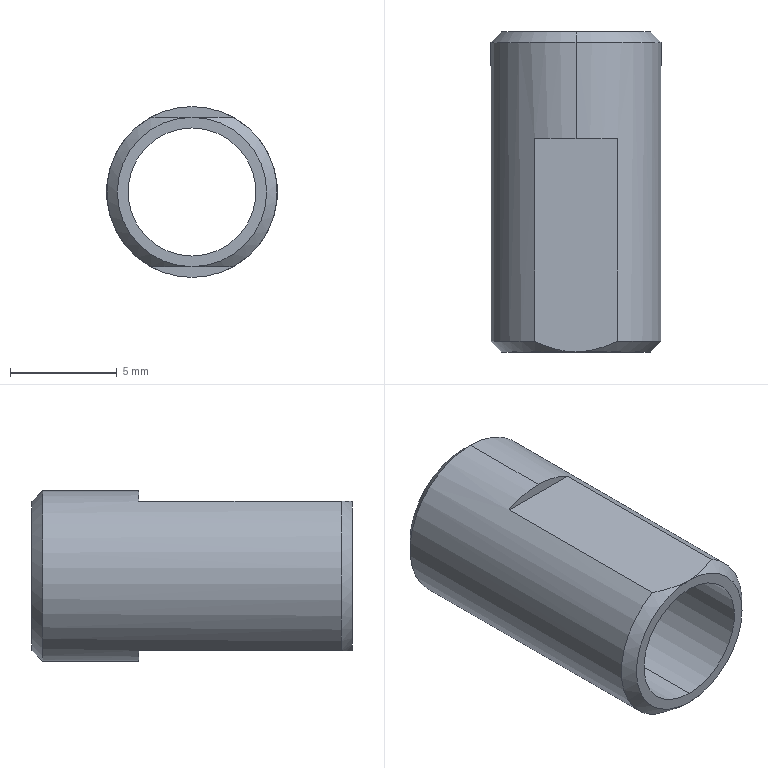Part | STEP file | 0246_214_Pin | 1 solid | 14 faces | box 8 x 15 x 8 mm | volume 298.54 mm3 | plane 6 | cylinder 4 | cone 4 | commonest cylinder face diameters 6 x2 8 x2
STEP:
#1=CARTESIAN_POINT('',(0.,0.,0.));
#2=DIRECTION('',(0.,0.,1.));
#3=DIRECTION('',(1.,0.,0.));
#4=AXIS2_PLACEMENT_3D('',#1,#2,#3);
#5=CARTESIAN_POINT('',(0.,0.,3.));
#6=VERTEX_POINT('',#5);
#7=CARTESIAN_POINT('',(0.,15.,3.));
#8=VERTEX_POINT('',#7);
#9=CARTESIAN_POINT('',(0.,15.,3.));
#10=DIRECTION('',(0.,1.,0.));
#11=VECTOR('',#10,1.);
#12=LINE('',#9,#11);
#13=CARTESIAN_POINT('',(0.,15.,0.));
#14=DIRECTION('',(0.,1.,0.));
#15=DIRECTION('',(0.,0.,1.));
#16=AXIS2_PLACEMENT_3D('',#13,#14,#15);
#17=CYLINDRICAL_SURFACE('',#16,3.);
#18=CARTESIAN_POINT('',(6.283,0.));
#19=DIRECTION('',(0.,1.));
#20=VECTOR('',#19,1.);
#21=LINE('',#18,#20);
#22=(GEOMETRIC_REPRESENTATION_CONTEXT(2)PARAMETRIC_REPRESENTATION_CONTEXT()REPRESENTATION_CONTEXT('',''));
#23=DEFINITIONAL_REPRESENTATION('',(#21),#22);
#24=PCURVE('',#17,#23);
#25=CARTESIAN_POINT('',(0.,15.,0.));
#26=DIRECTION('',(0.,1.,0.));
#27=DIRECTION('',(0.,0.,1.));
#28=AXIS2_PLACEMENT_3D('',#25,#26,#27);
#29=CYLINDRICAL_SURFACE('',#28,3.);
#30=CARTESIAN_POINT('',(0.,0.));
#31=DIRECTION('',(0.,1.));
#32=VECTOR('',#31,1.);
#33=LINE('',#30,#32);
#34=(GEOMETRIC_REPRESENTATION_CONTEXT(2)PARAMETRIC_REPRESENTATION_CONTEXT()REPRESENTATION_CONTEXT('',''));
#35=DEFINITIONAL_REPRESENTATION('',(#33),#34);
#36=PCURVE('',#29,#35);
#37=SURFACE_CURVE('',#12,(#24,#36),.PCURVE_S1.);
#38=EDGE_CURVE('',#6,#8,#37,.T.);
#39=ORIENTED_EDGE('',*,*,#38,.T.);
#40=CARTESIAN_POINT('',(0.,15.,-3.));
#41=VERTEX_POINT('',#40);
#42=CARTESIAN_POINT('',(0.,15.,0.));
#43=DIRECTION('',(0.,1.,0.));
#44=DIRECTION('',(0.,0.,1.));
#45=AXIS2_PLACEMENT_3D('',#42,#43,#44);
#46=CIRCLE('',#45,3.);
#47=CARTESIAN_POINT('',(0.,0.));
#48=DIRECTION('',(1.,0.));
#49=VECTOR('',#48,1.);
#50=LINE('',#47,#49);
#51=(GEOMETRIC_REPRESENTATION_CONTEXT(2)PARAMETRIC_REPRESENTATION_CONTEXT()REPRESENTATION_CONTEXT('',''));
#52=DEFINITIONAL_REPRESENTATION('',(#50),#51);
#53=PCURVE('',#17,#52);
#54=CARTESIAN_POINT('',(4.,15.,0.));
#55=DIRECTION('',(0.,1.,0.));
#56=DIRECTION('',(0.,0.,1.));
#57=AXIS2_PLACEMENT_3D('',#54,#55,#56);
#58=PLANE('',#57);
#59=CARTESIAN_POINT('',(0.,-4.));
#60=DIRECTION('',(1.,0.));
#61=AXIS2_PLACEMENT_2D('',#59,#60);
#62=CIRCLE('',#61,3.);
#63=(GEOMETRIC_REPRESENTATION_CONTEXT(2)PARAMETRIC_REPRESENTATION_CONTEXT()REPRESENTATION_CONTEXT('',''));
#64=DEFINITIONAL_REPRESENTATION('',(#62),#63);
#65=PCURVE('',#58,#64);
#66=SURFACE_CURVE('',#46,(#53,#65),.PCURVE_S1.);
#67=EDGE_CURVE('',#41,#8,#66,.T.);
#68=ORIENTED_EDGE('',*,*,#67,.F.);
#69=CARTESIAN_POINT('',(0.,0.,-3.));
#70=VERTEX_POINT('',#69);
#71=CARTESIAN_POINT('',(0.,15.,-3.));
#72=DIRECTION('',(0.,1.,0.));
#73=VECTOR('',#72,1.);
#74=LINE('',#71,#73);
#75=CARTESIAN_POINT('',(3.142,0.));
#76=DIRECTION('',(0.,1.));
#77=VECTOR('',#76,1.);
#78=LINE('',#75,#77);
#79=(GEOMETRIC_REPRESENTATION_CONTEXT(2)PARAMETRIC_REPRESENTATION_CONTEXT()REPRESENTATION_CONTEXT('',''));
#80=DEFINITIONAL_REPRESENTATION('',(#78),#79);
#81=PCURVE('',#17,#80);
#82=CARTESIAN_POINT('',(3.142,0.));
#83=DIRECTION('',(0.,1.));
#84=VECTOR('',#83,1.);
#85=LINE('',#82,#84);
#86=(GEOMETRIC_REPRESENTATION_CONTEXT(2)PARAMETRIC_REPRESENTATION_CONTEXT()REPRESENTATION_CONTEXT('',''));
#87=DEFINITIONAL_REPRESENTATION('',(#85),#86);
#88=PCURVE('',#29,#87);
#89=SURFACE_CURVE('',#74,(#81,#88),.PCURVE_S1.);
#90=EDGE_CURVE('',#70,#41,#89,.T.);
#91=ORIENTED_EDGE('',*,*,#90,.F.);
#92=CARTESIAN_POINT('',(0.,0.,0.));
#93=DIRECTION('',(0.,1.,0.));
#94=DIRECTION('',(0.,0.,1.));
#95=AXIS2_PLACEMENT_3D('',#92,#93,#94);
#96=CIRCLE('',#95,3.);
#97=CARTESIAN_POINT('',(0.,-15.));
#98=DIRECTION('',(1.,0.));
#99=VECTOR('',#98,1.);
#100=LINE('',#97,#99);
#101=(GEOMETRIC_REPRESENTATION_CONTEXT(2)PARAMETRIC_REPRESENTATION_CONTEXT()REPRESENTATION_CONTEXT('',''));
#102=DEFINITIONAL_REPRESENTATION('',(#100),#101);
#103=PCURVE('',#17,#102);
#104=CARTESIAN_POINT('',(4.,0.,0.));
#105=DIRECTION('',(0.,-1.,0.));
#106=DIRECTION('',(0.,0.,-1.));
#107=AXIS2_PLACEMENT_3D('',#104,#105,#106);
#108=PLANE('',#107);
#109=CARTESIAN_POINT('',(-3.,-4.));
#110=CARTESIAN_POINT('',(-3.,1.196));
#111=CARTESIAN_POINT('',(1.5,-1.402));
#112=CARTESIAN_POINT('',(6.,-4.));
#113=CARTESIAN_POINT('',(1.5,-6.598));
#114=CARTESIAN_POINT('',(-3.,-9.196));
#115=CARTESIAN_POINT('',(-3.,-4.));
#116=(BOUNDED_CURVE()B_SPLINE_CURVE(2,(#109,#110,#111,#112,#113,#114,#115),.UNSPECIFIED.,.T.,.F.)B_SPLINE_CURVE_WITH_KNOTS((1,2,2,2,2,1),(-2.094,0.,2.094,4.189,6.283,8.378),.UNSPECIFIED.)CURVE()GEOMETRIC_REPRESENTATION_ITEM()RATIONAL_B_SPLINE_CURVE((1.,0.5,1.,0.5,1.,0.5,1.))REPRESENTATION_ITEM(''));
#117=(GEOMETRIC_REPRESENTATION_CONTEXT(2)PARAMETRIC_REPRESENTATION_CONTEXT()REPRESENTATION_CONTEXT('',''));
#118=DEFINITIONAL_REPRESENTATION('',(#116),#117);
#119=PCURVE('',#108,#118);
#120=SURFACE_CURVE('',#96,(#103,#119),.PCURVE_S1.);
#121=EDGE_CURVE('',#70,#6,#120,.T.);
#122=ORIENTED_EDGE('',*,*,#121,.T.);
#123=EDGE_LOOP('',(#39,#68,#91,#122));
#124=FACE_BOUND('',#123,.F.);
#125=ADVANCED_FACE('',(#124),#17,.F.);
#126=CARTESIAN_POINT('',(0.,0.,-3.5));
#127=VERTEX_POINT('',#126);
#128=CARTESIAN_POINT('',(0.,0.,3.5));
#129=VERTEX_POINT('',#128);
#130=CARTESIAN_POINT('',(0.,0.,0.));
#131=DIRECTION('',(0.,-1.,0.));
#132=DIRECTION('',(0.,0.,-1.));
#133=AXIS2_PLACEMENT_3D('',#130,#131,#132);
#134=CIRCLE('',#133,3.5);
#135=CARTESIAN_POINT('',(0.,0.5,0.));
#136=DIRECTION('',(0.,1.,0.));
#137=DIRECTION('',(0.,0.,1.));
#138=AXIS2_PLACEMENT_3D('',#135,#136,#137);
#139=CONICAL_SURFACE('',#138,4.,0.7854);
#140=CARTESIAN_POINT('',(3.142,-0.5));
#141=DIRECTION('',(-1.,0.));
#142=VECTOR('',#141,1.);
#143=LINE('',#140,#142);
#144=(GEOMETRIC_REPRESENTATION_CONTEXT(2)PARAMETRIC_REPRESENTATION_CONTEXT()REPRESENTATION_CONTEXT('',''));
#145=DEFINITIONAL_REPRESENTATION('',(#143),#144);
#146=PCURVE('',#139,#145);
#147=CARTESIAN_POINT('',(0.,-4.));
#148=DIRECTION('',(1.,0.));
#149=AXIS2_PLACEMENT_2D('',#147,#148);
#150=CIRCLE('',#149,3.5);
#151=(GEOMETRIC_REPRESENTATION_CONTEXT(2)PARAMETRIC_REPRESENTATION_CONTEXT()REPRESENTATION_CONTEXT('',''));
#152=DEFINITIONAL_REPRESENTATION('',(#150),#151);
#153=PCURVE('',#108,#152);
#154=SURFACE_CURVE('',#134,(#146,#153),.PCURVE_S1.);
#155=EDGE_CURVE('',#127,#129,#154,.T.);
#156=ORIENTED_EDGE('',*,*,#155,.F.);
#157=CARTESIAN_POINT('',(0.,0.0008249,-3.501));
#158=VERTEX_POINT('',#157);
#159=CARTESIAN_POINT('',(0.,0.5,-4.));
#160=DIRECTION('',(0.,0.7071,-0.7071));
#161=VECTOR('',#160,1.);
#162=LINE('',#159,#161);
#163=CARTESIAN_POINT('',(3.142,0.));
#164=DIRECTION('',(0.,1.));
#165=VECTOR('',#164,1.);
#166=LINE('',#163,#165);
#167=(GEOMETRIC_REPRESENTATION_CONTEXT(2)PARAMETRIC_REPRESENTATION_CONTEXT()REPRESENTATION_CONTEXT('',''));
#168=DEFINITIONAL_REPRESENTATION('',(#166),#167);
#169=PCURVE('',#139,#168);
#170=CARTESIAN_POINT('',(0.,0.5,0.));
#171=DIRECTION('',(0.,1.,0.));
#172=DIRECTION('',(0.,0.,1.));
#173=AXIS2_PLACEMENT_3D('',#170,#171,#172);
#174=CONICAL_SURFACE('',#173,4.,0.7854);
#175=CARTESIAN_POINT('',(3.142,0.));
#176=DIRECTION('',(0.,1.));
#177=VECTOR('',#176,1.);
#178=LINE('',#175,#177);
#179=(GEOMETRIC_REPRESENTATION_CONTEXT(2)PARAMETRIC_REPRESENTATION_CONTEXT()REPRESENTATION_CONTEXT('',''));
#180=DEFINITIONAL_REPRESENTATION('',(#178),#179);
#181=PCURVE('',#174,#180);
#182=SURFACE_CURVE('',#162,(#169,#181),.PCURVE_S1.);
#183=EDGE_CURVE('',#127,#158,#182,.T.);
#184=ORIENTED_EDGE('',*,*,#183,.T.);
#185=CARTESIAN_POINT('',(1.935,0.5,-3.501));
#186=VERTEX_POINT('',#185);
#187=CARTESIAN_POINT('',(1.935,0.5,-3.501));
#188=CARTESIAN_POINT('',(1.785,0.4273,-3.501));
#189=CARTESIAN_POINT('',(1.631,0.3596,-3.501));
#190=CARTESIAN_POINT('',(1.317,0.2376,-3.501));
#191=CARTESIAN_POINT('',(1.156,0.1835,-3.501));
#192=CARTESIAN_POINT('',(0.6703,0.05077,-3.501));
#193=CARTESIAN_POINT('',(0.3396,0.0008249,-3.501));
#194=CARTESIAN_POINT('',(0.,0.0008249,-3.501));
#195=B_SPLINE_CURVE_WITH_KNOTS('',3,(#187,#188,#189,#190,#191,#192,#193,#194),.UNSPECIFIED.,.F.,.F.,(4,2,2,4),(0.002279,0.002778,0.003278,0.004277),.UNSPECIFIED.);
#196=CARTESIAN_POINT('',(2.637,0.));
#197=CARTESIAN_POINT('',(2.643,-0.01322));
#198=CARTESIAN_POINT('',(2.655,-0.03933));
#199=CARTESIAN_POINT('',(2.673,-0.07743));
#200=CARTESIAN_POINT('',(2.693,-0.1144));
#201=CARTESIAN_POINT('',(2.712,-0.1502));
#202=CARTESIAN_POINT('',(2.733,-0.1848));
#203=CARTESIAN_POINT('',(2.753,-0.2181));
#204=CARTESIAN_POINT('',(2.775,-0.25));
#205=CARTESIAN_POINT('',(2.797,-0.2803));
#206=CARTESIAN_POINT('',(2.819,-0.309));
#207=CARTESIAN_POINT('',(2.842,-0.336));
#208=CARTESIAN_POINT('',(2.865,-0.3611));
#209=CARTESIAN_POINT('',(2.888,-0.3842));
#210=CARTESIAN_POINT('',(2.912,-0.4055));
#211=CARTESIAN_POINT('',(2.937,-0.4247));
#212=CARTESIAN_POINT('',(2.961,-0.4418));
#213=CARTESIAN_POINT('',(2.986,-0.4569));
#214=CARTESIAN_POINT('',(3.012,-0.4697));
#215=CARTESIAN_POINT('',(3.037,-0.4803));
#216=CARTESIAN_POINT('',(3.063,-0.4887));
#217=CARTESIAN_POINT('',(3.089,-0.4947));
#218=CARTESIAN_POINT('',(3.115,-0.4984));
#219=CARTESIAN_POINT('',(3.133,-0.4992));
#220=CARTESIAN_POINT('',(3.142,-0.4992));
#221=B_SPLINE_CURVE_WITH_KNOTS('',3,(#196,#197,#198,#199,#200,#201,#202,#203,#204,#205,#206,#207,#208,#209,#210,#211,#212,#213,#214,#215,#216,#217,#218,#219,#220),.UNSPECIFIED.,.F.,.F.,(4,1,1,1,1,1,1,1,1,1,1,1,1,1,1,1,1,1,1,1,1,1,4),(0.002279,0.00237,0.002461,0.002551,0.002642,0.002733,0.002824,0.002915,0.003006,0.003096,0.003187,0.003278,0.003369,0.00346,0.003551,0.003641,0.003732,0.003823,0.003914,0.004005,0.004096,0.004186,0.004277),.QUASI_UNIFORM_KNOTS.);
#222=(GEOMETRIC_REPRESENTATION_CONTEXT(2)PARAMETRIC_REPRESENTATION_CONTEXT()REPRESENTATION_CONTEXT('',''));
#223=DEFINITIONAL_REPRESENTATION('',(#221),#222);
#224=PCURVE('',#139,#223);
#225=CARTESIAN_POINT('',(-1.935,10.,-3.501));
#226=DIRECTION('',(0.,0.,1.));
#227=DIRECTION('',(1.,0.,0.));
#228=AXIS2_PLACEMENT_3D('',#225,#226,#227);
#229=PLANE('',#228);
#230=CARTESIAN_POINT('',(3.87,-9.5));
#231=CARTESIAN_POINT('',(3.72,-9.573));
#232=CARTESIAN_POINT('',(3.566,-9.64));
#233=CARTESIAN_POINT('',(3.252,-9.762));
#234=CARTESIAN_POINT('',(3.091,-9.817));
#235=CARTESIAN_POINT('',(2.605,-9.949));
#236=CARTESIAN_POINT('',(2.275,-9.999));
#237=CARTESIAN_POINT('',(1.935,-9.999));
#238=B_SPLINE_CURVE_WITH_KNOTS('',3,(#230,#231,#232,#233,#234,#235,#236,#237),.UNSPECIFIED.,.F.,.F.,(4,2,2,4),(0.002279,0.002778,0.003278,0.004277),.UNSPECIFIED.);
#239=(GEOMETRIC_REPRESENTATION_CONTEXT(2)PARAMETRIC_REPRESENTATION_CONTEXT()REPRESENTATION_CONTEXT('',''));
#240=DEFINITIONAL_REPRESENTATION('',(#238),#239);
#241=PCURVE('',#229,#240);
#242=SURFACE_CURVE('',#195,(#224,#241),.PCURVE_S1.);
#243=EDGE_CURVE('',#186,#158,#242,.T.);
#244=ORIENTED_EDGE('',*,*,#243,.F.);
#245=CARTESIAN_POINT('',(1.935,0.5,3.501));
#246=VERTEX_POINT('',#245);
#247=CARTESIAN_POINT('',(0.,0.5,0.));
#248=DIRECTION('',(0.,1.,0.));
#249=DIRECTION('',(0.,0.,-1.));
#250=AXIS2_PLACEMENT_3D('',#247,#248,#249);
#251=CIRCLE('',#250,4.);
#252=CARTESIAN_POINT('',(-3.142,0.));
#253=DIRECTION('',(1.,0.));
#254=VECTOR('',#253,1.);
#255=LINE('',#252,#254);
#256=(GEOMETRIC_REPRESENTATION_CONTEXT(2)PARAMETRIC_REPRESENTATION_CONTEXT()REPRESENTATION_CONTEXT('',''));
#257=DEFINITIONAL_REPRESENTATION('',(#255),#256);
#258=PCURVE('',#139,#257);
#259=CARTESIAN_POINT('',(0.,15.,0.));
#260=DIRECTION('',(0.,1.,0.));
#261=DIRECTION('',(0.,0.,1.));
#262=AXIS2_PLACEMENT_3D('',#259,#260,#261);
#263=CYLINDRICAL_SURFACE('',#262,4.);
#264=CARTESIAN_POINT('',(-3.142,-14.5));
#265=DIRECTION('',(1.,0.));
#266=VECTOR('',#265,1.);
#267=LINE('',#264,#266);
#268=(GEOMETRIC_REPRESENTATION_CONTEXT(2)PARAMETRIC_REPRESENTATION_CONTEXT()REPRESENTATION_CONTEXT('',''));
#269=DEFINITIONAL_REPRESENTATION('',(#267),#268);
#270=PCURVE('',#263,#269);
#271=SURFACE_CURVE('',#251,(#258,#270),.PCURVE_S1.);
#272=EDGE_CURVE('',#246,#186,#271,.T.);
#273=ORIENTED_EDGE('',*,*,#272,.F.);
#274=CARTESIAN_POINT('',(0.,0.0008249,3.501));
#275=VERTEX_POINT('',#274);
#276=CARTESIAN_POINT('',(0.,0.0008249,3.501));
#277=CARTESIAN_POINT('',(0.3396,0.0008249,3.501));
#278=CARTESIAN_POINT('',(0.6703,0.05077,3.501));
#279=CARTESIAN_POINT('',(1.156,0.1835,3.501));
#280=CARTESIAN_POINT('',(1.317,0.2376,3.501));
#281=CARTESIAN_POINT('',(1.631,0.3596,3.501));
#282=CARTESIAN_POINT('',(1.785,0.4273,3.501));
#283=CARTESIAN_POINT('',(1.935,0.5,3.501));
#284=B_SPLINE_CURVE_WITH_KNOTS('',3,(#276,#277,#278,#279,#280,#281,#282,#283),.UNSPECIFIED.,.F.,.F.,(4,2,2,4),(0.004536,0.005536,0.006036,0.006535),.UNSPECIFIED.);
#285=CARTESIAN_POINT('',(0.,-0.4992));
#286=CARTESIAN_POINT('',(0.008818,-0.4992));
#287=CARTESIAN_POINT('',(0.02641,-0.4984));
#288=CARTESIAN_POINT('',(0.05264,-0.4947));
#289=CARTESIAN_POINT('',(0.07868,-0.4887));
#290=CARTESIAN_POINT('',(0.1045,-0.4803));
#291=CARTESIAN_POINT('',(0.1301,-0.4697));
#292=CARTESIAN_POINT('',(0.1553,-0.4569));
#293=CARTESIAN_POINT('',(0.1803,-0.4418));
#294=CARTESIAN_POINT('',(0.205,-0.4247));
#295=CARTESIAN_POINT('',(0.2293,-0.4055));
#296=CARTESIAN_POINT('',(0.2532,-0.3842));
#297=CARTESIAN_POINT('',(0.2768,-0.3611));
#298=CARTESIAN_POINT('',(0.2999,-0.336));
#299=CARTESIAN_POINT('',(0.3227,-0.309));
#300=CARTESIAN_POINT('',(0.345,-0.2803));
#301=CARTESIAN_POINT('',(0.3669,-0.25));
#302=CARTESIAN_POINT('',(0.3882,-0.2181));
#303=CARTESIAN_POINT('',(0.409,-0.1848));
#304=CARTESIAN_POINT('',(0.4293,-0.1502));
#305=CARTESIAN_POINT('',(0.449,-0.1144));
#306=CARTESIAN_POINT('',(0.4682,-0.07743));
#307=CARTESIAN_POINT('',(0.4868,-0.03933));
#308=CARTESIAN_POINT('',(0.499,-0.01322));
#309=CARTESIAN_POINT('',(0.5049,0.));
#310=B_SPLINE_CURVE_WITH_KNOTS('',3,(#285,#286,#287,#288,#289,#290,#291,#292,#293,#294,#295,#296,#297,#298,#299,#300,#301,#302,#303,#304,#305,#306,#307,#308,#309),.UNSPECIFIED.,.F.,.F.,(4,1,1,1,1,1,1,1,1,1,1,1,1,1,1,1,1,1,1,1,1,1,4),(0.004536,0.004627,0.004718,0.004809,0.004899,0.00499,0.005081,0.005172,0.005263,0.005354,0.005445,0.005536,0.005627,0.005717,0.005808,0.005899,0.00599,0.006081,0.006172,0.006263,0.006354,0.006444,0.006535),.QUASI_UNIFORM_KNOTS.);
#311=(GEOMETRIC_REPRESENTATION_CONTEXT(2)PARAMETRIC_REPRESENTATION_CONTEXT()REPRESENTATION_CONTEXT('',''));
#312=DEFINITIONAL_REPRESENTATION('',(#310),#311);
#313=PCURVE('',#139,#312);
#314=CARTESIAN_POINT('',(-1.935,10.,3.501));
#315=DIRECTION('',(0.,0.,-1.));
#316=DIRECTION('',(-1.,0.,0.));
#317=AXIS2_PLACEMENT_3D('',#314,#315,#316);
#318=PLANE('',#317);
#319=CARTESIAN_POINT('',(-1.935,-9.999));
#320=CARTESIAN_POINT('',(-2.275,-9.999));
#321=CARTESIAN_POINT('',(-2.605,-9.949));
#322=CARTESIAN_POINT('',(-3.091,-9.817));
#323=CARTESIAN_POINT('',(-3.252,-9.762));
#324=CARTESIAN_POINT('',(-3.566,-9.64));
#325=CARTESIAN_POINT('',(-3.72,-9.573));
#326=CARTESIAN_POINT('',(-3.87,-9.5));
#327=B_SPLINE_CURVE_WITH_KNOTS('',3,(#319,#320,#321,#322,#323,#324,#325,#326),.UNSPECIFIED.,.F.,.F.,(4,2,2,4),(0.004536,0.005536,0.006036,0.006535),.UNSPECIFIED.);
#328=(GEOMETRIC_REPRESENTATION_CONTEXT(2)PARAMETRIC_REPRESENTATION_CONTEXT()REPRESENTATION_CONTEXT('',''));
#329=DEFINITIONAL_REPRESENTATION('',(#327),#328);
#330=PCURVE('',#318,#329);
#331=SURFACE_CURVE('',#284,(#313,#330),.PCURVE_S1.);
#332=EDGE_CURVE('',#275,#246,#331,.T.);
#333=ORIENTED_EDGE('',*,*,#332,.F.);
#334=CARTESIAN_POINT('',(0.,0.5,4.));
#335=DIRECTION('',(0.,0.7071,0.7071));
#336=VECTOR('',#335,1.);
#337=LINE('',#334,#336);
#338=CARTESIAN_POINT('',(0.,0.));
#339=DIRECTION('',(0.,1.));
#340=VECTOR('',#339,1.);
#341=LINE('',#338,#340);
#342=(GEOMETRIC_REPRESENTATION_CONTEXT(2)PARAMETRIC_REPRESENTATION_CONTEXT()REPRESENTATION_CONTEXT('',''));
#343=DEFINITIONAL_REPRESENTATION('',(#341),#342);
#344=PCURVE('',#139,#343);
#345=CARTESIAN_POINT('',(6.283,0.));
#346=DIRECTION('',(0.,1.));
#347=VECTOR('',#346,1.);
#348=LINE('',#345,#347);
#349=(GEOMETRIC_REPRESENTATION_CONTEXT(2)PARAMETRIC_REPRESENTATION_CONTEXT()REPRESENTATION_CONTEXT('',''));
#350=DEFINITIONAL_REPRESENTATION('',(#348),#349);
#351=PCURVE('',#174,#350);
#352=SURFACE_CURVE('',#337,(#344,#351),.PCURVE_S1.);
#353=EDGE_CURVE('',#129,#275,#352,.T.);
#354=ORIENTED_EDGE('',*,*,#353,.F.);
#355=EDGE_LOOP('',(#156,#184,#244,#273,#333,#354));
#356=FACE_BOUND('',#355,.T.);
#357=ADVANCED_FACE('',(#356),#139,.T.);
#358=CARTESIAN_POINT('',(0.,15.,3.5));
#359=VERTEX_POINT('',#358);
#360=CARTESIAN_POINT('',(0.,15.,-3.5));
#361=VERTEX_POINT('',#360);
#362=CARTESIAN_POINT('',(0.,15.,0.));
#363=DIRECTION('',(0.,1.,0.));
#364=DIRECTION('',(0.,0.,1.));
#365=AXIS2_PLACEMENT_3D('',#362,#363,#364);
#366=CIRCLE('',#365,3.5);
#367=CARTESIAN_POINT('',(0.,15.,0.));
#368=DIRECTION('',(0.,-1.,0.));
#369=DIRECTION('',(0.,0.,-1.));
#370=AXIS2_PLACEMENT_3D('',#367,#368,#369);
#371=CONICAL_SURFACE('',#370,3.5,0.7854);
#372=CARTESIAN_POINT('',(3.142,0.));
#373=DIRECTION('',(-1.,0.));
#374=VECTOR('',#373,1.);
#375=LINE('',#372,#374);
#376=(GEOMETRIC_REPRESENTATION_CONTEXT(2)PARAMETRIC_REPRESENTATION_CONTEXT()REPRESENTATION_CONTEXT('',''));
#377=DEFINITIONAL_REPRESENTATION('',(#375),#376);
#378=PCURVE('',#371,#377);
#379=CARTESIAN_POINT('',(0.,-4.));
#380=DIRECTION('',(1.,0.));
#381=AXIS2_PLACEMENT_2D('',#379,#380);
#382=CIRCLE('',#381,3.5);
#383=(GEOMETRIC_REPRESENTATION_CONTEXT(2)PARAMETRIC_REPRESENTATION_CONTEXT()REPRESENTATION_CONTEXT('',''));
#384=DEFINITIONAL_REPRESENTATION('',(#382),#383);
#385=PCURVE('',#58,#384);
#386=SURFACE_CURVE('',#366,(#378,#385),.PCURVE_S1.);
#387=EDGE_CURVE('',#359,#361,#386,.T.);
#388=ORIENTED_EDGE('',*,*,#387,.F.);
#389=CARTESIAN_POINT('',(0.,14.5,4.));
#390=VERTEX_POINT('',#389);
#391=CARTESIAN_POINT('',(0.,15.,3.5));
#392=DIRECTION('',(0.,-0.7071,0.7071));
#393=VECTOR('',#392,1.);
#394=LINE('',#391,#393);
#395=CARTESIAN_POINT('',(3.142,0.));
#396=DIRECTION('',(0.,1.));
#397=VECTOR('',#396,1.);
#398=LINE('',#395,#397);
#399=(GEOMETRIC_REPRESENTATION_CONTEXT(2)PARAMETRIC_REPRESENTATION_CONTEXT()REPRESENTATION_CONTEXT('',''));
#400=DEFINITIONAL_REPRESENTATION('',(#398),#399);
#401=PCURVE('',#371,#400);
#402=CARTESIAN_POINT('',(0.,15.,0.));
#403=DIRECTION('',(0.,-1.,0.));
#404=DIRECTION('',(0.,0.,-1.));
#405=AXIS2_PLACEMENT_3D('',#402,#403,#404);
#406=CONICAL_SURFACE('',#405,3.5,0.7854);
#407=CARTESIAN_POINT('',(3.142,0.));
#408=DIRECTION('',(0.,1.));
#409=VECTOR('',#408,1.);
#410=LINE('',#407,#409);
#411=(GEOMETRIC_REPRESENTATION_CONTEXT(2)PARAMETRIC_REPRESENTATION_CONTEXT()REPRESENTATION_CONTEXT('',''));
#412=DEFINITIONAL_REPRESENTATION('',(#410),#411);
#413=PCURVE('',#406,#412);
#414=SURFACE_CURVE('',#394,(#401,#413),.PCURVE_S1.);
#415=EDGE_CURVE('',#359,#390,#414,.T.);
#416=ORIENTED_EDGE('',*,*,#415,.T.);
#417=CARTESIAN_POINT('',(0.,14.5,-4.));
#418=VERTEX_POINT('',#417);
#419=CARTESIAN_POINT('',(0.,14.5,0.));
#420=DIRECTION('',(0.,-1.,0.));
#421=DIRECTION('',(0.,0.,1.));
#422=AXIS2_PLACEMENT_3D('',#419,#420,#421);
#423=CIRCLE('',#422,4.);
#424=CARTESIAN_POINT('',(-3.142,0.5));
#425=DIRECTION('',(1.,0.));
#426=VECTOR('',#425,1.);
#427=LINE('',#424,#426);
#428=(GEOMETRIC_REPRESENTATION_CONTEXT(2)PARAMETRIC_REPRESENTATION_CONTEXT()REPRESENTATION_CONTEXT('',''));
#429=DEFINITIONAL_REPRESENTATION('',(#427),#428);
#430=PCURVE('',#371,#429);
#431=CARTESIAN_POINT('',(6.283,-0.5));
#432=DIRECTION('',(-1.,0.));
#433=VECTOR('',#432,1.);
#434=LINE('',#431,#433);
#435=(GEOMETRIC_REPRESENTATION_CONTEXT(2)PARAMETRIC_REPRESENTATION_CONTEXT()REPRESENTATION_CONTEXT('',''));
#436=DEFINITIONAL_REPRESENTATION('',(#434),#435);
#437=PCURVE('',#263,#436);
#438=SURFACE_CURVE('',#423,(#430,#437),.PCURVE_S1.);
#439=EDGE_CURVE('',#418,#390,#438,.T.);
#440=ORIENTED_EDGE('',*,*,#439,.F.);
#441=CARTESIAN_POINT('',(0.,15.,-3.5));
#442=DIRECTION('',(0.,-0.7071,-0.7071));
#443=VECTOR('',#442,1.);
#444=LINE('',#441,#443);
#445=CARTESIAN_POINT('',(0.,0.));
#446=DIRECTION('',(0.,1.));
#447=VECTOR('',#446,1.);
#448=LINE('',#445,#447);
#449=(GEOMETRIC_REPRESENTATION_CONTEXT(2)PARAMETRIC_REPRESENTATION_CONTEXT()REPRESENTATION_CONTEXT('',''));
#450=DEFINITIONAL_REPRESENTATION('',(#448),#449);
#451=PCURVE('',#371,#450);
#452=CARTESIAN_POINT('',(6.283,0.));
#453=DIRECTION('',(0.,1.));
#454=VECTOR('',#453,1.);
#455=LINE('',#452,#454);
#456=(GEOMETRIC_REPRESENTATION_CONTEXT(2)PARAMETRIC_REPRESENTATION_CONTEXT()REPRESENTATION_CONTEXT('',''));
#457=DEFINITIONAL_REPRESENTATION('',(#455),#456);
#458=PCURVE('',#406,#457);
#459=SURFACE_CURVE('',#444,(#451,#458),.PCURVE_S1.);
#460=EDGE_CURVE('',#361,#418,#459,.T.);
#461=ORIENTED_EDGE('',*,*,#460,.F.);
#462=EDGE_LOOP('',(#388,#416,#440,#461));
#463=FACE_BOUND('',#462,.T.);
#464=ADVANCED_FACE('',(#463),#371,.T.);
#465=CARTESIAN_POINT('',(0.,10.,-4.));
#466=VERTEX_POINT('',#465);
#467=CARTESIAN_POINT('',(1.935,10.,-3.501));
#468=VERTEX_POINT('',#467);
#469=CARTESIAN_POINT('',(0.,10.,0.));
#470=DIRECTION('',(0.,-1.,0.));
#471=DIRECTION('',(1.,0.,0.));
#472=AXIS2_PLACEMENT_3D('',#469,#470,#471);
#473=CIRCLE('',#472,4.);
#474=CARTESIAN_POINT('',(7.854,-5.));
#475=DIRECTION('',(-1.,0.));
#476=VECTOR('',#475,1.);
#477=LINE('',#474,#476);
#478=(GEOMETRIC_REPRESENTATION_CONTEXT(2)PARAMETRIC_REPRESENTATION_CONTEXT()REPRESENTATION_CONTEXT('',''));
#479=DEFINITIONAL_REPRESENTATION('',(#477),#478);
#480=PCURVE('',#263,#479);
#481=CARTESIAN_POINT('',(0.,10.,0.));
#482=DIRECTION('',(0.,-1.,0.));
#483=DIRECTION('',(1.,0.,0.));
#484=AXIS2_PLACEMENT_3D('',#481,#482,#483);
#485=PLANE('',#484);
#486=CARTESIAN_POINT('',(0.,0.));
#487=DIRECTION('',(1.,0.));
#488=AXIS2_PLACEMENT_2D('',#486,#487);
#489=CIRCLE('',#488,4.);
#490=(GEOMETRIC_REPRESENTATION_CONTEXT(2)PARAMETRIC_REPRESENTATION_CONTEXT()REPRESENTATION_CONTEXT('',''));
#491=DEFINITIONAL_REPRESENTATION('',(#489),#490);
#492=PCURVE('',#485,#491);
#493=SURFACE_CURVE('',#473,(#480,#492),.PCURVE_S1.);
#494=EDGE_CURVE('',#466,#468,#493,.T.);
#495=ORIENTED_EDGE('',*,*,#494,.F.);
#496=CARTESIAN_POINT('',(0.,15.,-4.));
#497=DIRECTION('',(0.,1.,0.));
#498=VECTOR('',#497,1.);
#499=LINE('',#496,#498);
#500=CARTESIAN_POINT('',(3.142,0.));
#501=DIRECTION('',(0.,1.));
#502=VECTOR('',#501,1.);
#503=LINE('',#500,#502);
#504=(GEOMETRIC_REPRESENTATION_CONTEXT(2)PARAMETRIC_REPRESENTATION_CONTEXT()REPRESENTATION_CONTEXT('',''));
#505=DEFINITIONAL_REPRESENTATION('',(#503),#504);
#506=PCURVE('',#263,#505);
#507=CARTESIAN_POINT('',(0.,15.,0.));
#508=DIRECTION('',(0.,1.,0.));
#509=DIRECTION('',(0.,0.,1.));
#510=AXIS2_PLACEMENT_3D('',#507,#508,#509);
#511=CYLINDRICAL_SURFACE('',#510,4.);
#512=CARTESIAN_POINT('',(3.142,0.));
#513=DIRECTION('',(0.,1.));
#514=VECTOR('',#513,1.);
#515=LINE('',#512,#514);
#516=(GEOMETRIC_REPRESENTATION_CONTEXT(2)PARAMETRIC_REPRESENTATION_CONTEXT()REPRESENTATION_CONTEXT('',''));
#517=DEFINITIONAL_REPRESENTATION('',(#515),#516);
#518=PCURVE('',#511,#517);
#519=SURFACE_CURVE('',#499,(#506,#518),.PCURVE_S1.);
#520=EDGE_CURVE('',#466,#418,#519,.T.);
#521=ORIENTED_EDGE('',*,*,#520,.T.);
#522=ORIENTED_EDGE('',*,*,#439,.T.);
#523=CARTESIAN_POINT('',(0.,10.,4.));
#524=VERTEX_POINT('',#523);
#525=CARTESIAN_POINT('',(0.,15.,4.));
#526=DIRECTION('',(0.,1.,0.));
#527=VECTOR('',#526,1.);
#528=LINE('',#525,#527);
#529=CARTESIAN_POINT('',(0.,0.));
#530=DIRECTION('',(0.,1.));
#531=VECTOR('',#530,1.);
#532=LINE('',#529,#531);
#533=(GEOMETRIC_REPRESENTATION_CONTEXT(2)PARAMETRIC_REPRESENTATION_CONTEXT()REPRESENTATION_CONTEXT('',''));
#534=DEFINITIONAL_REPRESENTATION('',(#532),#533);
#535=PCURVE('',#263,#534);
#536=CARTESIAN_POINT('',(6.283,0.));
#537=DIRECTION('',(0.,1.));
#538=VECTOR('',#537,1.);
#539=LINE('',#536,#538);
#540=(GEOMETRIC_REPRESENTATION_CONTEXT(2)PARAMETRIC_REPRESENTATION_CONTEXT()REPRESENTATION_CONTEXT('',''));
#541=DEFINITIONAL_REPRESENTATION('',(#539),#540);
#542=PCURVE('',#511,#541);
#543=SURFACE_CURVE('',#528,(#535,#542),.PCURVE_S1.);
#544=EDGE_CURVE('',#524,#390,#543,.T.);
#545=ORIENTED_EDGE('',*,*,#544,.F.);
#546=CARTESIAN_POINT('',(1.935,10.,3.501));
#547=VERTEX_POINT('',#546);
#548=CARTESIAN_POINT('',(0.,10.,0.));
#549=DIRECTION('',(0.,-1.,0.));
#550=DIRECTION('',(1.,0.,0.));
#551=AXIS2_PLACEMENT_3D('',#548,#549,#550);
#552=CIRCLE('',#551,4.);
#553=CARTESIAN_POINT('',(1.571,-5.));
#554=DIRECTION('',(-1.,0.));
#555=VECTOR('',#554,1.);
#556=LINE('',#553,#555);
#557=(GEOMETRIC_REPRESENTATION_CONTEXT(2)PARAMETRIC_REPRESENTATION_CONTEXT()REPRESENTATION_CONTEXT('',''));
#558=DEFINITIONAL_REPRESENTATION('',(#556),#557);
#559=PCURVE('',#263,#558);
#560=CARTESIAN_POINT('',(0.,10.,0.));
#561=DIRECTION('',(0.,-1.,0.));
#562=DIRECTION('',(1.,0.,0.));
#563=AXIS2_PLACEMENT_3D('',#560,#561,#562);
#564=PLANE('',#563);
#565=CARTESIAN_POINT('',(0.,0.));
#566=DIRECTION('',(1.,0.));
#567=AXIS2_PLACEMENT_2D('',#565,#566);
#568=CIRCLE('',#567,4.);
#569=(GEOMETRIC_REPRESENTATION_CONTEXT(2)PARAMETRIC_REPRESENTATION_CONTEXT()REPRESENTATION_CONTEXT('',''));
#570=DEFINITIONAL_REPRESENTATION('',(#568),#569);
#571=PCURVE('',#564,#570);
#572=SURFACE_CURVE('',#552,(#559,#571),.PCURVE_S1.);
#573=EDGE_CURVE('',#547,#524,#572,.T.);
#574=ORIENTED_EDGE('',*,*,#573,.F.);
#575=CARTESIAN_POINT('',(1.935,10.,3.501));
#576=DIRECTION('',(0.,-1.,0.));
#577=VECTOR('',#576,1.);
#578=LINE('',#575,#577);
#579=CARTESIAN_POINT('',(0.5049,-5.));
#580=DIRECTION('',(0.,-1.));
#581=VECTOR('',#580,1.);
#582=LINE('',#579,#581);
#583=(GEOMETRIC_REPRESENTATION_CONTEXT(2)PARAMETRIC_REPRESENTATION_CONTEXT()REPRESENTATION_CONTEXT('',''));
#584=DEFINITIONAL_REPRESENTATION('',(#582),#583);
#585=PCURVE('',#263,#584);
#586=CARTESIAN_POINT('',(-3.87,0.));
#587=DIRECTION('',(0.,-1.));
#588=VECTOR('',#587,1.);
#589=LINE('',#586,#588);
#590=(GEOMETRIC_REPRESENTATION_CONTEXT(2)PARAMETRIC_REPRESENTATION_CONTEXT()REPRESENTATION_CONTEXT('',''));
#591=DEFINITIONAL_REPRESENTATION('',(#589),#590);
#592=PCURVE('',#318,#591);
#593=SURFACE_CURVE('',#578,(#585,#592),.PCURVE_S1.);
#594=EDGE_CURVE('',#547,#246,#593,.T.);
#595=ORIENTED_EDGE('',*,*,#594,.T.);
#596=ORIENTED_EDGE('',*,*,#272,.T.);
#597=CARTESIAN_POINT('',(1.935,10.,-3.501));
#598=DIRECTION('',(0.,-1.,0.));
#599=VECTOR('',#598,1.);
#600=LINE('',#597,#599);
#601=CARTESIAN_POINT('',(2.637,-5.));
#602=DIRECTION('',(0.,-1.));
#603=VECTOR('',#602,1.);
#604=LINE('',#601,#603);
#605=(GEOMETRIC_REPRESENTATION_CONTEXT(2)PARAMETRIC_REPRESENTATION_CONTEXT()REPRESENTATION_CONTEXT('',''));
#606=DEFINITIONAL_REPRESENTATION('',(#604),#605);
#607=PCURVE('',#263,#606);
#608=CARTESIAN_POINT('',(3.87,0.));
#609=DIRECTION('',(0.,-1.));
#610=VECTOR('',#609,1.);
#611=LINE('',#608,#610);
#612=(GEOMETRIC_REPRESENTATION_CONTEXT(2)PARAMETRIC_REPRESENTATION_CONTEXT()REPRESENTATION_CONTEXT('',''));
#613=DEFINITIONAL_REPRESENTATION('',(#611),#612);
#614=PCURVE('',#229,#613);
#615=SURFACE_CURVE('',#600,(#607,#614),.PCURVE_S1.);
#616=EDGE_CURVE('',#468,#186,#615,.T.);
#617=ORIENTED_EDGE('',*,*,#616,.F.);
#618=EDGE_LOOP('',(#495,#521,#522,#545,#574,#595,#596,#617));
#619=FACE_BOUND('',#618,.T.);
#620=ADVANCED_FACE('',(#619),#263,.T.);
#621=CARTESIAN_POINT('',(0.,15.,0.));
#622=DIRECTION('',(0.,1.,0.));
#623=DIRECTION('',(0.,0.,1.));
#624=AXIS2_PLACEMENT_3D('',#621,#622,#623);
#625=CIRCLE('',#624,3.);
#626=CARTESIAN_POINT('',(0.,-4.));
#627=DIRECTION('',(1.,0.));
#628=AXIS2_PLACEMENT_2D('',#626,#627);
#629=CIRCLE('',#628,3.);
#630=(GEOMETRIC_REPRESENTATION_CONTEXT(2)PARAMETRIC_REPRESENTATION_CONTEXT()REPRESENTATION_CONTEXT('',''));
#631=DEFINITIONAL_REPRESENTATION('',(#629),#630);
#632=PCURVE('',#58,#631);
#633=CARTESIAN_POINT('',(0.,0.));
#634=DIRECTION('',(1.,0.));
#635=VECTOR('',#634,1.);
#636=LINE('',#633,#635);
#637=(GEOMETRIC_REPRESENTATION_CONTEXT(2)PARAMETRIC_REPRESENTATION_CONTEXT()REPRESENTATION_CONTEXT('',''));
#638=DEFINITIONAL_REPRESENTATION('',(#636),#637);
#639=PCURVE('',#29,#638);
#640=SURFACE_CURVE('',#625,(#632,#639),.PCURVE_S1.);
#641=EDGE_CURVE('',#8,#41,#640,.T.);
#642=ORIENTED_EDGE('',*,*,#641,.F.);
#643=ORIENTED_EDGE('',*,*,#67,.F.);
#644=EDGE_LOOP('',(#642,#643));
#645=FACE_BOUND('',#644,.T.);
#646=CARTESIAN_POINT('',(0.,15.,0.));
#647=DIRECTION('',(0.,1.,0.));
#648=DIRECTION('',(0.,0.,1.));
#649=AXIS2_PLACEMENT_3D('',#646,#647,#648);
#650=CIRCLE('',#649,3.5);
#651=CARTESIAN_POINT('',(0.,-4.));
#652=DIRECTION('',(1.,0.));
#653=AXIS2_PLACEMENT_2D('',#651,#652);
#654=CIRCLE('',#653,3.5);
#655=(GEOMETRIC_REPRESENTATION_CONTEXT(2)PARAMETRIC_REPRESENTATION_CONTEXT()REPRESENTATION_CONTEXT('',''));
#656=DEFINITIONAL_REPRESENTATION('',(#654),#655);
#657=PCURVE('',#58,#656);
#658=CARTESIAN_POINT('',(9.425,0.));
#659=DIRECTION('',(-1.,0.));
#660=VECTOR('',#659,1.);
#661=LINE('',#658,#660);
#662=(GEOMETRIC_REPRESENTATION_CONTEXT(2)PARAMETRIC_REPRESENTATION_CONTEXT()REPRESENTATION_CONTEXT('',''));
#663=DEFINITIONAL_REPRESENTATION('',(#661),#662);
#664=PCURVE('',#406,#663);
#665=SURFACE_CURVE('',#650,(#657,#664),.PCURVE_S1.);
#666=EDGE_CURVE('',#361,#359,#665,.T.);
#667=ORIENTED_EDGE('',*,*,#666,.T.);
#668=ORIENTED_EDGE('',*,*,#387,.T.);
#669=EDGE_LOOP('',(#667,#668));
#670=FACE_BOUND('',#669,.T.);
#671=ADVANCED_FACE('',(#645,#670),#58,.T.);
#672=ORIENTED_EDGE('',*,*,#520,.F.);
#673=CARTESIAN_POINT('',(-1.935,10.,-3.501));
#674=VERTEX_POINT('',#673);
#675=CARTESIAN_POINT('',(0.,10.,0.));
#676=DIRECTION('',(0.,-1.,0.));
#677=DIRECTION('',(1.,0.,0.));
#678=AXIS2_PLACEMENT_3D('',#675,#676,#677);
#679=CIRCLE('',#678,4.);
#680=CARTESIAN_POINT('',(7.854,-5.));
#681=DIRECTION('',(-1.,0.));
#682=VECTOR('',#681,1.);
#683=LINE('',#680,#682);
#684=(GEOMETRIC_REPRESENTATION_CONTEXT(2)PARAMETRIC_REPRESENTATION_CONTEXT()REPRESENTATION_CONTEXT('',''));
#685=DEFINITIONAL_REPRESENTATION('',(#683),#684);
#686=PCURVE('',#511,#685);
#687=CARTESIAN_POINT('',(0.,0.));
#688=DIRECTION('',(1.,0.));
#689=AXIS2_PLACEMENT_2D('',#687,#688);
#690=CIRCLE('',#689,4.);
#691=(GEOMETRIC_REPRESENTATION_CONTEXT(2)PARAMETRIC_REPRESENTATION_CONTEXT()REPRESENTATION_CONTEXT('',''));
#692=DEFINITIONAL_REPRESENTATION('',(#690),#691);
#693=PCURVE('',#485,#692);
#694=SURFACE_CURVE('',#679,(#686,#693),.PCURVE_S1.);
#695=EDGE_CURVE('',#674,#466,#694,.T.);
#696=ORIENTED_EDGE('',*,*,#695,.F.);
#697=CARTESIAN_POINT('',(-1.935,0.5,-3.501));
#698=VERTEX_POINT('',#697);
#699=CARTESIAN_POINT('',(-1.935,10.,-3.501));
#700=DIRECTION('',(0.,-1.,0.));
#701=VECTOR('',#700,1.);
#702=LINE('',#699,#701);
#703=CARTESIAN_POINT('',(3.647,-5.));
#704=DIRECTION('',(0.,-1.));
#705=VECTOR('',#704,1.);
#706=LINE('',#703,#705);
#707=(GEOMETRIC_REPRESENTATION_CONTEXT(2)PARAMETRIC_REPRESENTATION_CONTEXT()REPRESENTATION_CONTEXT('',''));
#708=DEFINITIONAL_REPRESENTATION('',(#706),#707);
#709=PCURVE('',#511,#708);
#710=CARTESIAN_POINT('',(0.,0.));
#711=DIRECTION('',(0.,-1.));
#712=VECTOR('',#711,1.);
#713=LINE('',#710,#712);
#714=(GEOMETRIC_REPRESENTATION_CONTEXT(2)PARAMETRIC_REPRESENTATION_CONTEXT()REPRESENTATION_CONTEXT('',''));
#715=DEFINITIONAL_REPRESENTATION('',(#713),#714);
#716=PCURVE('',#229,#715);
#717=SURFACE_CURVE('',#702,(#709,#716),.PCURVE_S1.);
#718=EDGE_CURVE('',#674,#698,#717,.T.);
#719=ORIENTED_EDGE('',*,*,#718,.T.);
#720=CARTESIAN_POINT('',(-1.935,0.5,3.501));
#721=VERTEX_POINT('',#720);
#722=CARTESIAN_POINT('',(0.,0.5,0.));
#723=DIRECTION('',(0.,1.,0.));
#724=DIRECTION('',(0.,0.,-1.));
#725=AXIS2_PLACEMENT_3D('',#722,#723,#724);
#726=CIRCLE('',#725,4.);
#727=CARTESIAN_POINT('',(3.142,-14.5));
#728=DIRECTION('',(1.,0.));
#729=VECTOR('',#728,1.);
#730=LINE('',#727,#729);
#731=(GEOMETRIC_REPRESENTATION_CONTEXT(2)PARAMETRIC_REPRESENTATION_CONTEXT()REPRESENTATION_CONTEXT('',''));
#732=DEFINITIONAL_REPRESENTATION('',(#730),#731);
#733=PCURVE('',#511,#732);
#734=CARTESIAN_POINT('',(3.142,0.));
#735=DIRECTION('',(1.,0.));
#736=VECTOR('',#735,1.);
#737=LINE('',#734,#736);
#738=(GEOMETRIC_REPRESENTATION_CONTEXT(2)PARAMETRIC_REPRESENTATION_CONTEXT()REPRESENTATION_CONTEXT('',''));
#739=DEFINITIONAL_REPRESENTATION('',(#737),#738);
#740=PCURVE('',#174,#739);
#741=SURFACE_CURVE('',#726,(#733,#740),.PCURVE_S1.);
#742=EDGE_CURVE('',#698,#721,#741,.T.);
#743=ORIENTED_EDGE('',*,*,#742,.T.);
#744=CARTESIAN_POINT('',(-1.935,10.,3.501));
#745=VERTEX_POINT('',#744);
#746=CARTESIAN_POINT('',(-1.935,10.,3.501));
#747=DIRECTION('',(0.,-1.,0.));
#748=VECTOR('',#747,1.);
#749=LINE('',#746,#748);
#750=CARTESIAN_POINT('',(5.778,-5.));
#751=DIRECTION('',(0.,-1.));
#752=VECTOR('',#751,1.);
#753=LINE('',#750,#752);
#754=(GEOMETRIC_REPRESENTATION_CONTEXT(2)PARAMETRIC_REPRESENTATION_CONTEXT()REPRESENTATION_CONTEXT('',''));
#755=DEFINITIONAL_REPRESENTATION('',(#753),#754);
#756=PCURVE('',#511,#755);
#757=CARTESIAN_POINT('',(0.,0.));
#758=DIRECTION('',(0.,-1.));
#759=VECTOR('',#758,1.);
#760=LINE('',#757,#759);
#761=(GEOMETRIC_REPRESENTATION_CONTEXT(2)PARAMETRIC_REPRESENTATION_CONTEXT()REPRESENTATION_CONTEXT('',''));
#762=DEFINITIONAL_REPRESENTATION('',(#760),#761);
#763=PCURVE('',#318,#762);
#764=SURFACE_CURVE('',#749,(#756,#763),.PCURVE_S1.);
#765=EDGE_CURVE('',#745,#721,#764,.T.);
#766=ORIENTED_EDGE('',*,*,#765,.F.);
#767=CARTESIAN_POINT('',(0.,10.,0.));
#768=DIRECTION('',(0.,-1.,0.));
#769=DIRECTION('',(1.,0.,0.));
#770=AXIS2_PLACEMENT_3D('',#767,#768,#769);
#771=CIRCLE('',#770,4.);
#772=CARTESIAN_POINT('',(7.854,-5.));
#773=DIRECTION('',(-1.,0.));
#774=VECTOR('',#773,1.);
#775=LINE('',#772,#774);
#776=(GEOMETRIC_REPRESENTATION_CONTEXT(2)PARAMETRIC_REPRESENTATION_CONTEXT()REPRESENTATION_CONTEXT('',''));
#777=DEFINITIONAL_REPRESENTATION('',(#775),#776);
#778=PCURVE('',#511,#777);
#779=CARTESIAN_POINT('',(0.,0.));
#780=DIRECTION('',(1.,0.));
#781=AXIS2_PLACEMENT_2D('',#779,#780);
#782=CIRCLE('',#781,4.);
#783=(GEOMETRIC_REPRESENTATION_CONTEXT(2)PARAMETRIC_REPRESENTATION_CONTEXT()REPRESENTATION_CONTEXT('',''));
#784=DEFINITIONAL_REPRESENTATION('',(#782),#783);
#785=PCURVE('',#564,#784);
#786=SURFACE_CURVE('',#771,(#778,#785),.PCURVE_S1.);
#787=EDGE_CURVE('',#524,#745,#786,.T.);
#788=ORIENTED_EDGE('',*,*,#787,.F.);
#789=ORIENTED_EDGE('',*,*,#544,.T.);
#790=CARTESIAN_POINT('',(0.,14.5,0.));
#791=DIRECTION('',(0.,-1.,0.));
#792=DIRECTION('',(0.,0.,1.));
#793=AXIS2_PLACEMENT_3D('',#790,#791,#792);
#794=CIRCLE('',#793,4.);
#795=CARTESIAN_POINT('',(6.283,-0.5));
#796=DIRECTION('',(-1.,0.));
#797=VECTOR('',#796,1.);
#798=LINE('',#795,#797);
#799=(GEOMETRIC_REPRESENTATION_CONTEXT(2)PARAMETRIC_REPRESENTATION_CONTEXT()REPRESENTATION_CONTEXT('',''));
#800=DEFINITIONAL_REPRESENTATION('',(#798),#799);
#801=PCURVE('',#511,#800);
#802=CARTESIAN_POINT('',(3.142,0.5));
#803=DIRECTION('',(1.,0.));
#804=VECTOR('',#803,1.);
#805=LINE('',#802,#804);
#806=(GEOMETRIC_REPRESENTATION_CONTEXT(2)PARAMETRIC_REPRESENTATION_CONTEXT()REPRESENTATION_CONTEXT('',''));
#807=DEFINITIONAL_REPRESENTATION('',(#805),#806);
#808=PCURVE('',#406,#807);
#809=SURFACE_CURVE('',#794,(#801,#808),.PCURVE_S1.);
#810=EDGE_CURVE('',#390,#418,#809,.T.);
#811=ORIENTED_EDGE('',*,*,#810,.T.);
#812=EDGE_LOOP('',(#672,#696,#719,#743,#766,#788,#789,#811));
#813=FACE_BOUND('',#812,.T.);
#814=ADVANCED_FACE('',(#813),#511,.T.);
#815=CARTESIAN_POINT('',(0.,0.,0.));
#816=DIRECTION('',(0.,1.,0.));
#817=DIRECTION('',(0.,0.,1.));
#818=AXIS2_PLACEMENT_3D('',#815,#816,#817);
#819=CIRCLE('',#818,3.);
#820=CARTESIAN_POINT('',(-3.,-4.));
#821=CARTESIAN_POINT('',(-3.,1.196));
#822=CARTESIAN_POINT('',(1.5,-1.402));
#823=CARTESIAN_POINT('',(6.,-4.));
#824=CARTESIAN_POINT('',(1.5,-6.598));
#825=CARTESIAN_POINT('',(-3.,-9.196));
#826=CARTESIAN_POINT('',(-3.,-4.));
#827=(BOUNDED_CURVE()B_SPLINE_CURVE(2,(#820,#821,#822,#823,#824,#825,#826),.UNSPECIFIED.,.T.,.F.)B_SPLINE_CURVE_WITH_KNOTS((1,2,2,2,2,1),(-2.094,0.,2.094,4.189,6.283,8.378),.UNSPECIFIED.)CURVE()GEOMETRIC_REPRESENTATION_ITEM()RATIONAL_B_SPLINE_CURVE((1.,0.5,1.,0.5,1.,0.5,1.))REPRESENTATION_ITEM(''));
#828=(GEOMETRIC_REPRESENTATION_CONTEXT(2)PARAMETRIC_REPRESENTATION_CONTEXT()REPRESENTATION_CONTEXT('',''));
#829=DEFINITIONAL_REPRESENTATION('',(#827),#828);
#830=PCURVE('',#108,#829);
#831=CARTESIAN_POINT('',(0.,-15.));
#832=DIRECTION('',(1.,0.));
#833=VECTOR('',#832,1.);
#834=LINE('',#831,#833);
#835=(GEOMETRIC_REPRESENTATION_CONTEXT(2)PARAMETRIC_REPRESENTATION_CONTEXT()REPRESENTATION_CONTEXT('',''));
#836=DEFINITIONAL_REPRESENTATION('',(#834),#835);
#837=PCURVE('',#29,#836);
#838=SURFACE_CURVE('',#819,(#830,#837),.PCURVE_S1.);
#839=EDGE_CURVE('',#6,#70,#838,.T.);
#840=ORIENTED_EDGE('',*,*,#839,.T.);
#841=ORIENTED_EDGE('',*,*,#121,.T.);
#842=EDGE_LOOP('',(#840,#841));
#843=FACE_BOUND('',#842,.T.);
#844=CARTESIAN_POINT('',(0.,0.,0.));
#845=DIRECTION('',(0.,-1.,0.));
#846=DIRECTION('',(0.,0.,-1.));
#847=AXIS2_PLACEMENT_3D('',#844,#845,#846);
#848=CIRCLE('',#847,3.5);
#849=CARTESIAN_POINT('',(0.,-4.));
#850=DIRECTION('',(1.,0.));
#851=AXIS2_PLACEMENT_2D('',#849,#850);
#852=CIRCLE('',#851,3.5);
#853=(GEOMETRIC_REPRESENTATION_CONTEXT(2)PARAMETRIC_REPRESENTATION_CONTEXT()REPRESENTATION_CONTEXT('',''));
#854=DEFINITIONAL_REPRESENTATION('',(#852),#853);
#855=PCURVE('',#108,#854);
#856=CARTESIAN_POINT('',(9.425,-0.5));
#857=DIRECTION('',(-1.,0.));
#858=VECTOR('',#857,1.);
#859=LINE('',#856,#858);
#860=(GEOMETRIC_REPRESENTATION_CONTEXT(2)PARAMETRIC_REPRESENTATION_CONTEXT()REPRESENTATION_CONTEXT('',''));
#861=DEFINITIONAL_REPRESENTATION('',(#859),#860);
#862=PCURVE('',#174,#861);
#863=SURFACE_CURVE('',#848,(#855,#862),.PCURVE_S1.);
#864=EDGE_CURVE('',#129,#127,#863,.T.);
#865=ORIENTED_EDGE('',*,*,#864,.T.);
#866=ORIENTED_EDGE('',*,*,#155,.T.);
#867=EDGE_LOOP('',(#865,#866));
#868=FACE_BOUND('',#867,.T.);
#869=ADVANCED_FACE('',(#843,#868),#108,.T.);
#870=ORIENTED_EDGE('',*,*,#415,.F.);
#871=ORIENTED_EDGE('',*,*,#666,.F.);
#872=ORIENTED_EDGE('',*,*,#460,.T.);
#873=ORIENTED_EDGE('',*,*,#810,.F.);
#874=EDGE_LOOP('',(#870,#871,#872,#873));
#875=FACE_BOUND('',#874,.T.);
#876=ADVANCED_FACE('',(#875),#406,.T.);
#877=ORIENTED_EDGE('',*,*,#183,.F.);
#878=ORIENTED_EDGE('',*,*,#864,.F.);
#879=ORIENTED_EDGE('',*,*,#353,.T.);
#880=CARTESIAN_POINT('',(-1.935,0.5,3.501));
#881=CARTESIAN_POINT('',(-1.634,0.3543,3.501));
#882=CARTESIAN_POINT('',(-1.317,0.2275,3.501));
#883=CARTESIAN_POINT('',(-0.6713,0.05105,3.501));
#884=CARTESIAN_POINT('',(-0.3394,0.0008249,3.501));
#885=CARTESIAN_POINT('',(0.,0.0008249,3.501));
#886=B_SPLINE_CURVE_WITH_KNOTS('',3,(#880,#881,#882,#883,#884,#885),.UNSPECIFIED.,.F.,.F.,(4,2,4),(0.002537,0.003537,0.004536),.UNSPECIFIED.);
#887=CARTESIAN_POINT('',(5.778,0.));
#888=CARTESIAN_POINT('',(5.784,-0.01324));
#889=CARTESIAN_POINT('',(5.796,-0.03942));
#890=CARTESIAN_POINT('',(5.815,-0.07767));
#891=CARTESIAN_POINT('',(5.834,-0.1148));
#892=CARTESIAN_POINT('',(5.854,-0.1507));
#893=CARTESIAN_POINT('',(5.875,-0.1854));
#894=CARTESIAN_POINT('',(5.895,-0.2186));
#895=CARTESIAN_POINT('',(5.917,-0.2504));
#896=CARTESIAN_POINT('',(5.938,-0.2806));
#897=CARTESIAN_POINT('',(5.961,-0.3092));
#898=CARTESIAN_POINT('',(5.983,-0.336));
#899=CARTESIAN_POINT('',(6.006,-0.361));
#900=CARTESIAN_POINT('',(6.03,-0.3842));
#901=CARTESIAN_POINT('',(6.054,-0.4054));
#902=CARTESIAN_POINT('',(6.078,-0.4246));
#903=CARTESIAN_POINT('',(6.103,-0.4417));
#904=CARTESIAN_POINT('',(6.128,-0.4568));
#905=CARTESIAN_POINT('',(6.153,-0.4696));
#906=CARTESIAN_POINT('',(6.179,-0.4803));
#907=CARTESIAN_POINT('',(6.204,-0.4887));
#908=CARTESIAN_POINT('',(6.231,-0.4947));
#909=CARTESIAN_POINT('',(6.257,-0.4984));
#910=CARTESIAN_POINT('',(6.274,-0.4992));
#911=CARTESIAN_POINT('',(6.283,-0.4992));
#912=B_SPLINE_CURVE_WITH_KNOTS('',3,(#887,#888,#889,#890,#891,#892,#893,#894,#895,#896,#897,#898,#899,#900,#901,#902,#903,#904,#905,#906,#907,#908,#909,#910,#911),.UNSPECIFIED.,.F.,.F.,(4,1,1,1,1,1,1,1,1,1,1,1,1,1,1,1,1,1,1,1,1,1,4),(0.002537,0.002628,0.002719,0.00281,0.002901,0.002991,0.003082,0.003173,0.003264,0.003355,0.003446,0.003537,0.003627,0.003718,0.003809,0.0039,0.003991,0.004082,0.004172,0.004263,0.004354,0.004445,0.004536),.QUASI_UNIFORM_KNOTS.);
#913=(GEOMETRIC_REPRESENTATION_CONTEXT(2)PARAMETRIC_REPRESENTATION_CONTEXT()REPRESENTATION_CONTEXT('',''));
#914=DEFINITIONAL_REPRESENTATION('',(#912),#913);
#915=PCURVE('',#174,#914);
#916=CARTESIAN_POINT('',(0.,-9.5));
#917=CARTESIAN_POINT('',(-0.3011,-9.646));
#918=CARTESIAN_POINT('',(-0.6178,-9.772));
#919=CARTESIAN_POINT('',(-1.264,-9.949));
#920=CARTESIAN_POINT('',(-1.596,-9.999));
#921=CARTESIAN_POINT('',(-1.935,-9.999));
#922=B_SPLINE_CURVE_WITH_KNOTS('',3,(#916,#917,#918,#919,#920,#921),.UNSPECIFIED.,.F.,.F.,(4,2,4),(0.002537,0.003537,0.004536),.UNSPECIFIED.);
#923=(GEOMETRIC_REPRESENTATION_CONTEXT(2)PARAMETRIC_REPRESENTATION_CONTEXT()REPRESENTATION_CONTEXT('',''));
#924=DEFINITIONAL_REPRESENTATION('',(#922),#923);
#925=PCURVE('',#318,#924);
#926=SURFACE_CURVE('',#886,(#915,#925),.PCURVE_S1.);
#927=EDGE_CURVE('',#721,#275,#926,.T.);
#928=ORIENTED_EDGE('',*,*,#927,.F.);
#929=ORIENTED_EDGE('',*,*,#742,.F.);
#930=CARTESIAN_POINT('',(0.,0.0008249,-3.501));
#931=CARTESIAN_POINT('',(-0.3394,0.0008249,-3.501));
#932=CARTESIAN_POINT('',(-0.6713,0.05105,-3.501));
#933=CARTESIAN_POINT('',(-1.317,0.2275,-3.501));
#934=CARTESIAN_POINT('',(-1.634,0.3543,-3.501));
#935=CARTESIAN_POINT('',(-1.935,0.5,-3.501));
#936=B_SPLINE_CURVE_WITH_KNOTS('',3,(#930,#931,#932,#933,#934,#935),.UNSPECIFIED.,.F.,.F.,(4,2,4),(0.004277,0.005276,0.006275),.UNSPECIFIED.);
#937=CARTESIAN_POINT('',(3.142,-0.4992));
#938=CARTESIAN_POINT('',(3.15,-0.4992));
#939=CARTESIAN_POINT('',(3.168,-0.4984));
#940=CARTESIAN_POINT('',(3.194,-0.4947));
#941=CARTESIAN_POINT('',(3.22,-0.4887));
#942=CARTESIAN_POINT('',(3.246,-0.4803));
#943=CARTESIAN_POINT('',(3.272,-0.4696));
#944=CARTESIAN_POINT('',(3.297,-0.4568));
#945=CARTESIAN_POINT('',(3.322,-0.4417));
#946=CARTESIAN_POINT('',(3.347,-0.4246));
#947=CARTESIAN_POINT('',(3.371,-0.4054));
#948=CARTESIAN_POINT('',(3.395,-0.3842));
#949=CARTESIAN_POINT('',(3.418,-0.361));
#950=CARTESIAN_POINT('',(3.441,-0.336));
#951=CARTESIAN_POINT('',(3.464,-0.3092));
#952=CARTESIAN_POINT('',(3.486,-0.2806));
#953=CARTESIAN_POINT('',(3.508,-0.2504));
#954=CARTESIAN_POINT('',(3.529,-0.2186));
#955=CARTESIAN_POINT('',(3.55,-0.1854));
#956=CARTESIAN_POINT('',(3.571,-0.1507));
#957=CARTESIAN_POINT('',(3.59,-0.1148));
#958=CARTESIAN_POINT('',(3.61,-0.07767));
#959=CARTESIAN_POINT('',(3.628,-0.03942));
#960=CARTESIAN_POINT('',(3.641,-0.01324));
#961=CARTESIAN_POINT('',(3.647,0.));
#962=B_SPLINE_CURVE_WITH_KNOTS('',3,(#937,#938,#939,#940,#941,#942,#943,#944,#945,#946,#947,#948,#949,#950,#951,#952,#953,#954,#955,#956,#957,#958,#959,#960,#961),.UNSPECIFIED.,.F.,.F.,(4,1,1,1,1,1,1,1,1,1,1,1,1,1,1,1,1,1,1,1,1,1,4),(0.004277,0.004368,0.004459,0.00455,0.00464,0.004731,0.004822,0.004913,0.005004,0.005094,0.005185,0.005276,0.005367,0.005458,0.005548,0.005639,0.00573,0.005821,0.005912,0.006002,0.006093,0.006184,0.006275),.QUASI_UNIFORM_KNOTS.);
#963=(GEOMETRIC_REPRESENTATION_CONTEXT(2)PARAMETRIC_REPRESENTATION_CONTEXT()REPRESENTATION_CONTEXT('',''));
#964=DEFINITIONAL_REPRESENTATION('',(#962),#963);
#965=PCURVE('',#174,#964);
#966=CARTESIAN_POINT('',(1.935,-9.999));
#967=CARTESIAN_POINT('',(1.596,-9.999));
#968=CARTESIAN_POINT('',(1.264,-9.949));
#969=CARTESIAN_POINT('',(0.6178,-9.772));
#970=CARTESIAN_POINT('',(0.3011,-9.646));
#971=CARTESIAN_POINT('',(0.,-9.5));
#972=B_SPLINE_CURVE_WITH_KNOTS('',3,(#966,#967,#968,#969,#970,#971),.UNSPECIFIED.,.F.,.F.,(4,2,4),(0.004277,0.005276,0.006275),.UNSPECIFIED.);
#973=(GEOMETRIC_REPRESENTATION_CONTEXT(2)PARAMETRIC_REPRESENTATION_CONTEXT()REPRESENTATION_CONTEXT('',''));
#974=DEFINITIONAL_REPRESENTATION('',(#972),#973);
#975=PCURVE('',#229,#974);
#976=SURFACE_CURVE('',#936,(#965,#975),.PCURVE_S1.);
#977=EDGE_CURVE('',#158,#698,#976,.T.);
#978=ORIENTED_EDGE('',*,*,#977,.F.);
#979=EDGE_LOOP('',(#877,#878,#879,#928,#929,#978));
#980=FACE_BOUND('',#979,.T.);
#981=ADVANCED_FACE('',(#980),#174,.T.);
#982=ORIENTED_EDGE('',*,*,#927,.T.);
#983=ORIENTED_EDGE('',*,*,#332,.T.);
#984=ORIENTED_EDGE('',*,*,#594,.F.);
#985=CARTESIAN_POINT('',(-1.935,10.,3.501));
#986=DIRECTION('',(1.,0.,0.));
#987=VECTOR('',#986,1.);
#988=LINE('',#985,#987);
#989=CARTESIAN_POINT('',(0.,0.));
#990=DIRECTION('',(-1.,0.));
#991=VECTOR('',#990,1.);
#992=LINE('',#989,#991);
#993=(GEOMETRIC_REPRESENTATION_CONTEXT(2)PARAMETRIC_REPRESENTATION_CONTEXT()REPRESENTATION_CONTEXT('',''));
#994=DEFINITIONAL_REPRESENTATION('',(#992),#993);
#995=PCURVE('',#318,#994);
#996=CARTESIAN_POINT('',(-1.935,3.501));
#997=DIRECTION('',(1.,0.));
#998=VECTOR('',#997,1.);
#999=LINE('',#996,#998);
#1000=(GEOMETRIC_REPRESENTATION_CONTEXT(2)PARAMETRIC_REPRESENTATION_CONTEXT()REPRESENTATION_CONTEXT('',''));
#1001=DEFINITIONAL_REPRESENTATION('',(#999),#1000);
#1002=PCURVE('',#564,#1001);
#1003=SURFACE_CURVE('',#988,(#995,#1002),.PCURVE_S1.);
#1004=EDGE_CURVE('',#745,#547,#1003,.T.);
#1005=ORIENTED_EDGE('',*,*,#1004,.F.);
#1006=ORIENTED_EDGE('',*,*,#765,.T.);
#1007=EDGE_LOOP('',(#982,#983,#984,#1005,#1006));
#1008=FACE_BOUND('',#1007,.T.);
#1009=ADVANCED_FACE('',(#1008),#318,.F.);
#1010=ORIENTED_EDGE('',*,*,#573,.T.);
#1011=ORIENTED_EDGE('',*,*,#787,.T.);
#1012=ORIENTED_EDGE('',*,*,#1004,.T.);
#1013=EDGE_LOOP('',(#1010,#1011,#1012));
#1014=FACE_BOUND('',#1013,.T.);
#1015=ADVANCED_FACE('',(#1014),#564,.T.);
#1016=ORIENTED_EDGE('',*,*,#243,.T.);
#1017=ORIENTED_EDGE('',*,*,#977,.T.);
#1018=ORIENTED_EDGE('',*,*,#718,.F.);
#1019=CARTESIAN_POINT('',(-1.935,10.,-3.501));
#1020=DIRECTION('',(-1.,0.,0.));
#1021=VECTOR('',#1020,1.);
#1022=LINE('',#1019,#1021);
#1023=CARTESIAN_POINT('',(0.,0.));
#1024=DIRECTION('',(-1.,0.));
#1025=VECTOR('',#1024,1.);
#1026=LINE('',#1023,#1025);
#1027=(GEOMETRIC_REPRESENTATION_CONTEXT(2)PARAMETRIC_REPRESENTATION_CONTEXT()REPRESENTATION_CONTEXT('',''));
#1028=DEFINITIONAL_REPRESENTATION('',(#1026),#1027);
#1029=PCURVE('',#229,#1028);
#1030=CARTESIAN_POINT('',(-1.935,-3.501));
#1031=DIRECTION('',(-1.,0.));
#1032=VECTOR('',#1031,1.);
#1033=LINE('',#1030,#1032);
#1034=(GEOMETRIC_REPRESENTATION_CONTEXT(2)PARAMETRIC_REPRESENTATION_CONTEXT()REPRESENTATION_CONTEXT('',''));
#1035=DEFINITIONAL_REPRESENTATION('',(#1033),#1034);
#1036=PCURVE('',#485,#1035);
#1037=SURFACE_CURVE('',#1022,(#1029,#1036),.PCURVE_S1.);
#1038=EDGE_CURVE('',#468,#674,#1037,.T.);
#1039=ORIENTED_EDGE('',*,*,#1038,.F.);
#1040=ORIENTED_EDGE('',*,*,#616,.T.);
#1041=EDGE_LOOP('',(#1016,#1017,#1018,#1039,#1040));
#1042=FACE_BOUND('',#1041,.T.);
#1043=ADVANCED_FACE('',(#1042),#229,.F.);
#1044=ORIENTED_EDGE('',*,*,#695,.T.);
#1045=ORIENTED_EDGE('',*,*,#494,.T.);
#1046=ORIENTED_EDGE('',*,*,#1038,.T.);
#1047=EDGE_LOOP('',(#1044,#1045,#1046));
#1048=FACE_BOUND('',#1047,.T.);
#1049=ADVANCED_FACE('',(#1048),#485,.T.);
#1050=ORIENTED_EDGE('',*,*,#641,.F.);
#1051=ORIENTED_EDGE('',*,*,#38,.F.);
#1052=ORIENTED_EDGE('',*,*,#839,.T.);
#1053=ORIENTED_EDGE('',*,*,#90,.T.);
#1054=EDGE_LOOP('',(#1050,#1051,#1052,#1053));
#1055=FACE_BOUND('',#1054,.F.);
#1056=ADVANCED_FACE('',(#1055),#29,.F.);
#1057=CLOSED_SHELL('',(#125,#357,#464,#620,#671,#814,#869,#876,#981,#1009,#1015,#1043,#1049,#1056));
#1058=MANIFOLD_SOLID_BREP('',#1057);
#1059=(LENGTH_UNIT()NAMED_UNIT(*)SI_UNIT(.MILLI.,.METRE.));
#1060=UNCERTAINTY_MEASURE_WITH_UNIT(LENGTH_MEASURE(0.00002),#1059,'','');
#1061=(NAMED_UNIT(*)PLANE_ANGLE_UNIT()SI_UNIT($,.RADIAN.));
#1062=(NAMED_UNIT(*)SI_UNIT($,.STERADIAN.)SOLID_ANGLE_UNIT());
#1063=(GEOMETRIC_REPRESENTATION_CONTEXT(3)GLOBAL_UNCERTAINTY_ASSIGNED_CONTEXT((#1060))GLOBAL_UNIT_ASSIGNED_CONTEXT((#1059,#1061,#1062))REPRESENTATION_CONTEXT('',''));
#1064=ADVANCED_BREP_SHAPE_REPRESENTATION('',(#4,#1058),#1063);